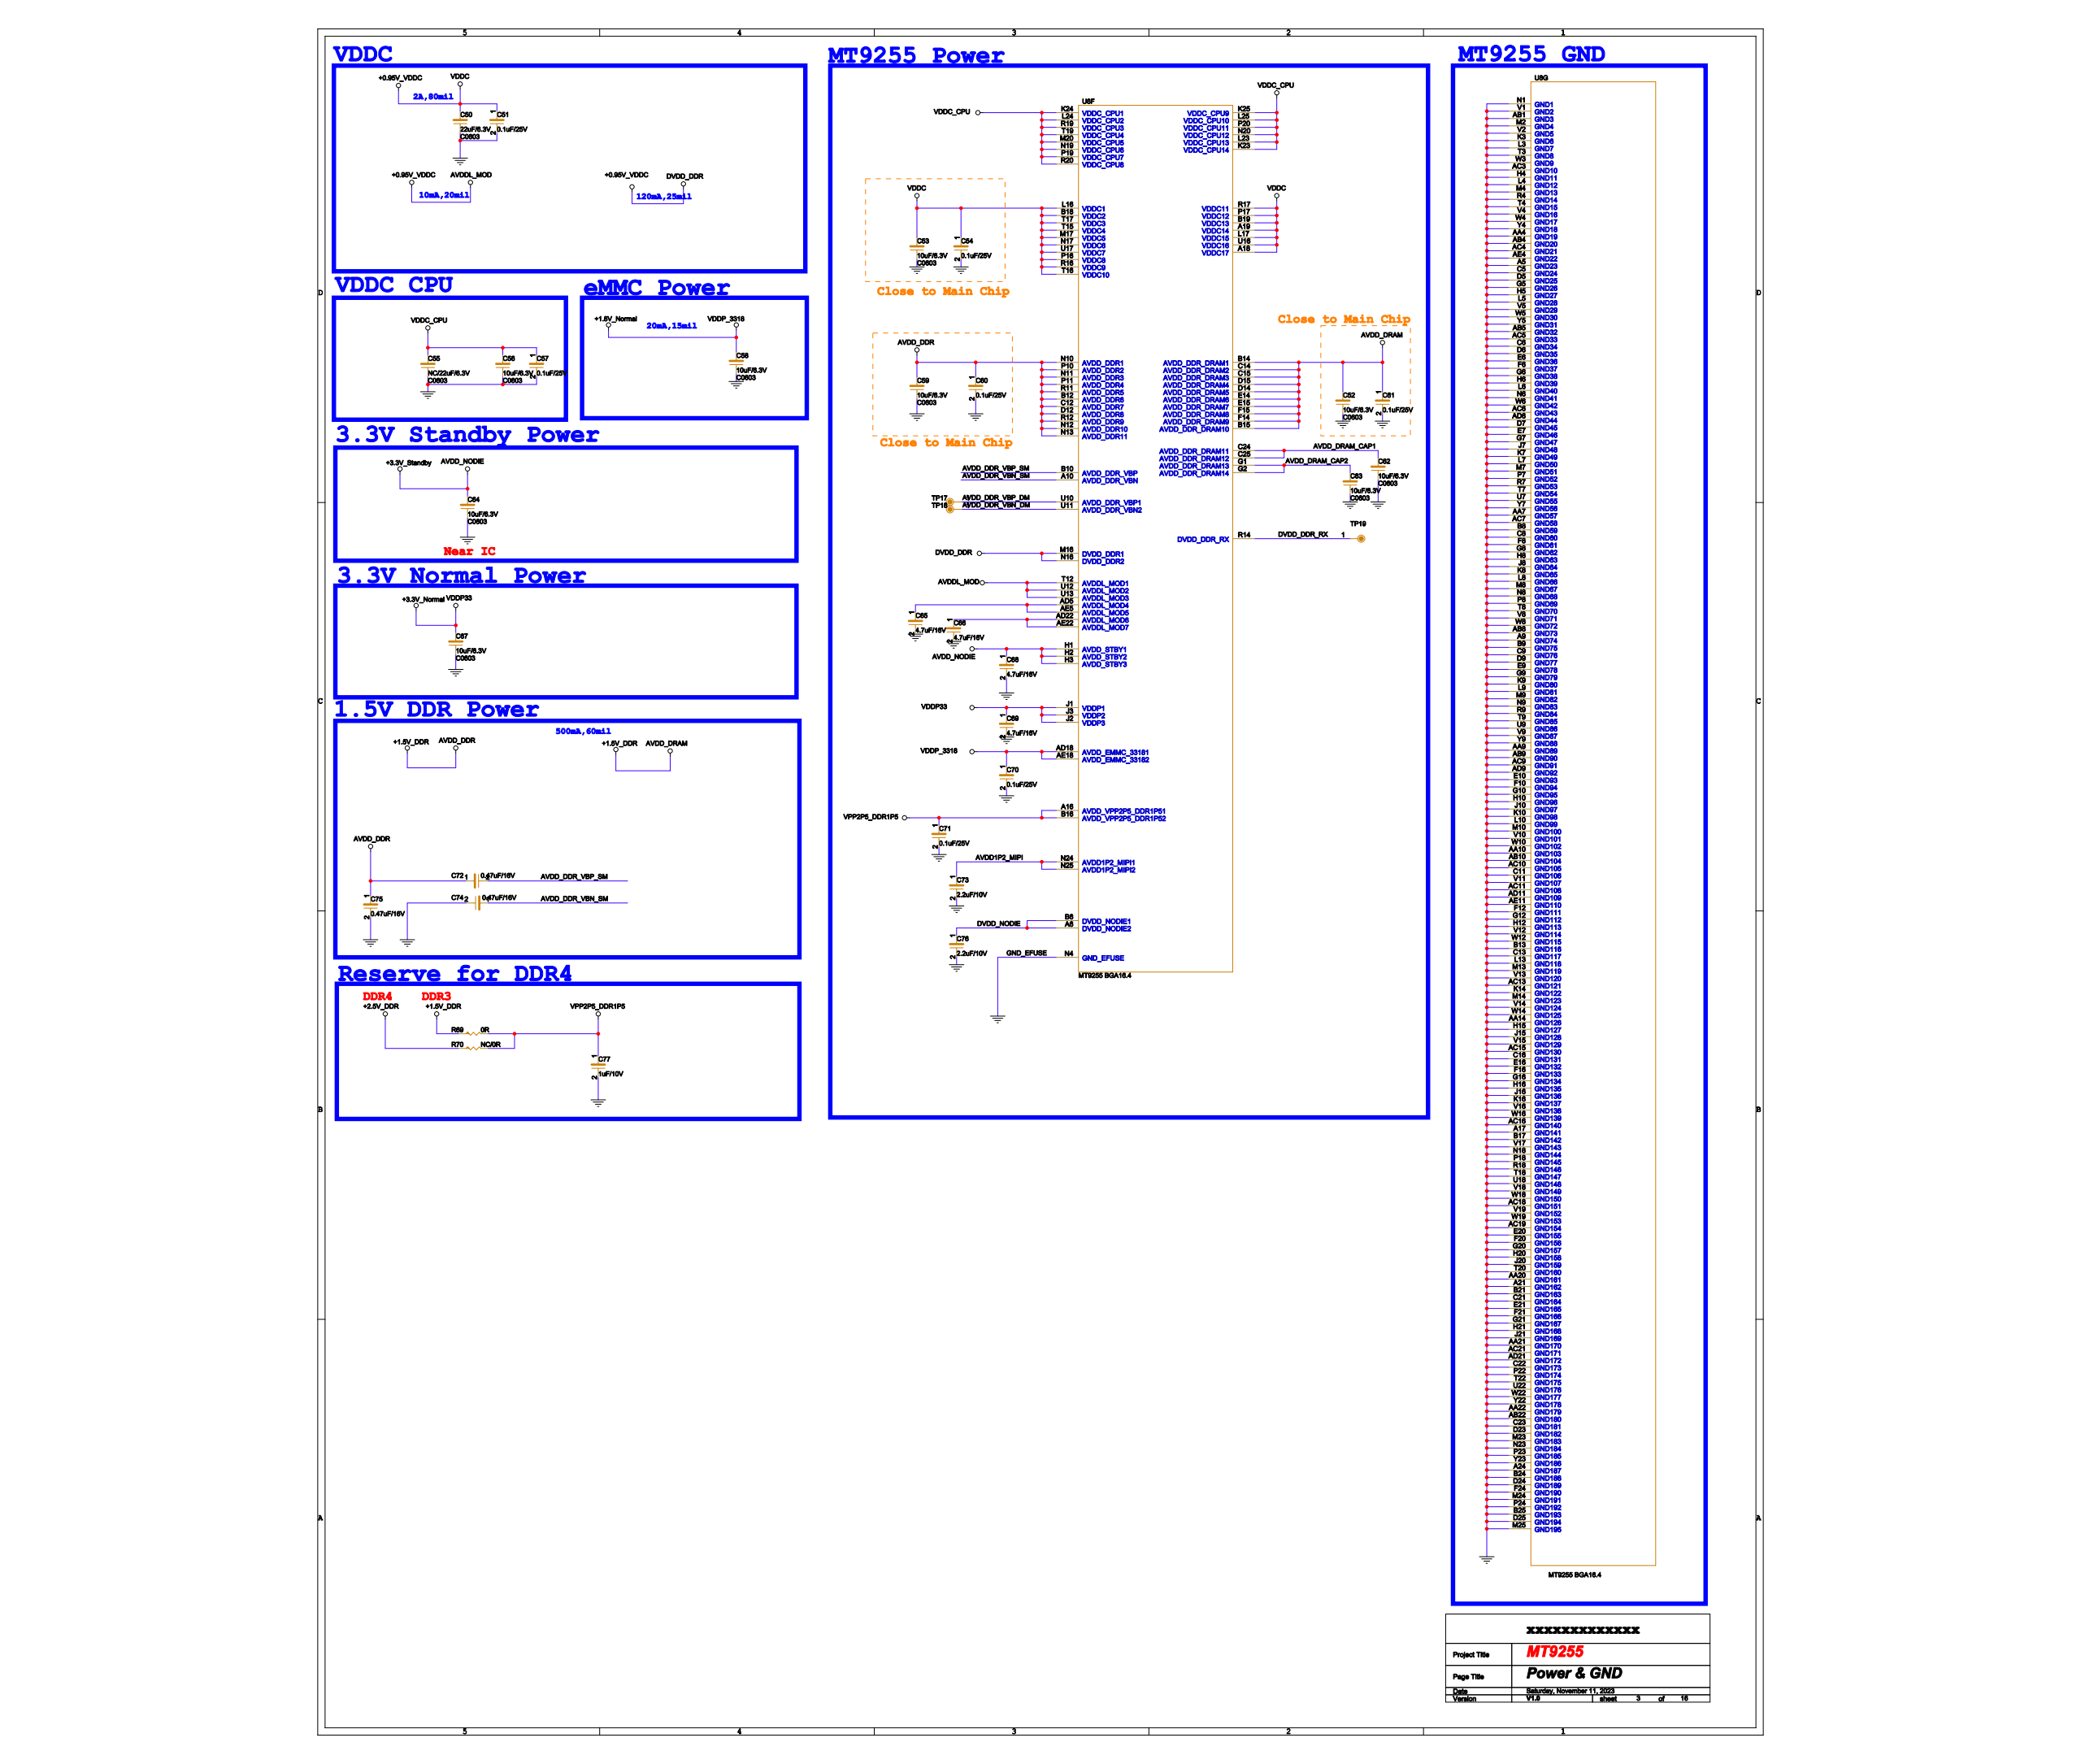Circuit board | Cadence Allegro | 1223 parts | 777 nets | one sheet of the schematic
Parts on this sheet (reference | value | footprint):
C50 | 22uF/6.3V | C0603
C51 | 0.1uF/25V | C0402
C52 | 10uF/6.3V | C0603
C53 | 10uF/6.3V | C0603
C54 | 0.1uF/25V | C0402
C55 | NC/22uF/6.3V | C0603
C56 | 10uF/6.3V | C0603
C57 | 0.1uF/25V | C0402
C58 | 10uF/6.3V | C0603
C59 | 10uF/6.3V | C0603
C60 | 0.1uF/25V | C0402
C61 | 0.1uF/25V | C0402
C62 | 10uF/6.3V | C0603
C63 | 10uF/6.3V | C0603
C64 | 10uF/6.3V | C0603
C65 | 4.7uF/16V | C0603
C66 | 4.7uF/16V | C0603
C67 | 10uF/6.3V | C0603
C68 | 4.7uF/16V | C0603
C69 | 4.7uF/16V | C0603
C70 | 0.1uF/25V | C0402
C71 | 0.1uF/25V | C0402
C72 | 0.47uF/16V | C0402
C73 | 2.2uF/10V | C0402
C74 | 0.47uF/16V | C0402
C75 | 0.47uF/16V | C0402
C76 | 2.2uF/10V | C0402
C77 | 1uF/10V | C0402
R69 | 0R | R0402
R70 | NC/0R | R0402
TP17 | DEO | TP06MM
TP18 | DEO | TP06MM
TP19 | DEO | TP06MM
U8 | MT9255 BGA16.4 | LFBGA462
U10 | EMMC_B153_2L | BGA153_13R00X11R50X0R90_2L
U16 | NTP8810 | QFN32_5X5MM
Nets of these parts (net: part-pin ...):
GND: C50-2 C51-2 C52-2 C53-2 C54-2 C55-2 C56-2 C57-2 C58-2 C59-2 C60-2 C61-2 C62-2 C63-2 C64-2 C65-2 C66-2 C67-2 C68-2 C69-2 C70-2 C71-2 C73-2 C74-2 C75-2 C76-2 C77-2 U8-A5 U8-A9 U8-A17 U8-A21 U8-A24 U8-AA4 U8-AA7 U8-AA9 U8-AA10 U8-AA14 U8-AA20 U8-AA21 U8-AA22 U8-AB1 U8-AB4 U8-AB5 U8-AB8 U8-AB9 U8-AB10 U8-AB22 U8-AC3 U8-AC4 U8-AC5 U8-AC6 U8-AC7 U8-AC9 U8-AC10 U8-AC11 U8-AC13 U8-AC15 U8-AC16 U8-AC18 U8-AC19 U8-AC21 U8-AD6 U8-AD9 U8-AD11 U8-AD21 U8-AE4 U8-AE11 U8-B8 U8-B9 U8-B13 U8-B17 U8-B21 U8-B24 U8-B25 U8-C5 U8-C6 U8-C8 U8-C9 U8-C11 U8-C13 U8-C16 U8-C21 U8-C22 U8-C23 U8-D5 U8-D6 U8-D7 U8-D9 U8-D23 U8-D24 U8-D25 U8-E6 U8-E7 U8-E9 U8-E10 U8-E16 U8-E20 U8-E21 U8-F6 U8-F8 U8-F10 U8-F12 U8-F16 U8-F20 U8-F21 U8-F24 U8-G5 U8-G6 U8-G7 U8-G8 U8-G9 U8-G10 U8-G12 U8-G16 U8-G20 U8-G21 U8-H4 U8-H5 U8-H6 U8-H8 U8-H10 U8-H12 U8-H15 U8-H16 U8-H20 U8-H21 U8-J7 U8-J8 U8-J10 U8-J15 U8-J16 U8-J20 U8-J21 U8-K3 U8-K7 U8-K8 U8-K9 U8-K10 U8-K14 U8-K16 U8-L3 U8-L4 U8-L5 U8-L6 U8-L7 U8-L8 U8-L9 U8-L10 U8-L13 U8-M2 U8-M4 U8-M7 U8-M8 U8-M9 U8-M10 U8-M13 U8-M14 U8-M23 U8-M24 U8-M25 U8-N1 U8-N4 U8-N6 U8-N8 U8-N9 U8-N18 U8-N23 U8-P7 U8-P8 U8-P18 U8-P22 U8-P23 U8-P24 U8-R4 U8-R7 U8-R9 U8-R18 U8-T3 U8-T4 U8-T7 U8-T8 U8-T9 U8-T18 U8-T20 U8-T22 U8-U7 U8-U9 U8-U18 U8-U22 U8-V1 U8-V2 U8-V4 U8-V5 U8-V8 U8-V9 U8-V10 U8-V11 U8-V12 U8-V13 U8-V14 U8-V15 U8-V16 U8-V17 U8-V18 U8-V19 U8-W3 U8-W4 U8-W5 U8-W6 U8-W8 U8-W10 U8-W12 U8-W14 U8-W16 U8-W18 U8-W19 U8-W22 U8-Y4 U8-Y5 U8-Y7 U8-Y9 U8-Y22 U8-Y23 U10-A6 U10-E7 U10-G5 U10-H10 U10-K8 U16-4
+3.3V_STANDBY: C64-1 C68-1 U8-H1 U8-H2 U8-H3
+1.5V_DDR: C52-1 C59-1 C60-1 C61-1 C72-1 C75-1 R69-1 U8-B12 U8-B14 U8-B15 U8-C12 U8-C14 U8-C15 U8-D12 U8-D14 U8-D15 U8-E14 U8-E15 U8-F14 U8-F15 U8-N10 U8-N11 U8-N12 U8-N13 U8-P10 U8-P11 U8-R11 U8-R12
+0.95V_VDDC: C50-1 C51-1 C53-1 C54-1 U8-A18 U8-A19 U8-B18 U8-B19 U8-L16 U8-L17 U8-M16 U8-M17 U8-N16 U8-N17 U8-P16 U8-P17 U8-R16 U8-R17 U8-T12 U8-T15 U8-T16 U8-T17 U8-U12 U8-U13 U8-U16 U8-U17
VDDC_CPU: C55-1 C56-1 C57-1 U8-K23 U8-K24 U8-K25 U8-L23 U8-L24 U8-L25 U8-M20 U8-N19 U8-N20 U8-P19 U8-P20 U8-R19 U8-R20 U8-T19
+3.3V_EMMC: C67-1 C69-1 U8-J1 U8-J2 U8-J3 U10-E6 U10-J10 U10-K9
+1.8V_NORMAL: C58-1 C70-1 U8-AD18 U8-AE18 U10-C6 U10-M4 U10-N4
VPP2P5_DDR1P5: C71-1 C77-1 R69-2 R70-2 U8-A16 U8-B16
+2.5V_DDR: R70-1
AVDD_DRAM_CAP1: C62-1 U8-C24 U8-C25
AVDD_DRAM_CAP2: C63-1 U8-G1 U8-G2
N185692934: C65-1 U8-AD5 U8-AE5
N185692958: C66-1 U8-AD22 U8-AE22
AVDD_DDR_VBP_SM: C72-2 U8-B10
AVDD_DDR_VBN_SM: C74-1 U8-A10
AVDD1P2_MIPI: C73-1 U8-N24 U8-N25
DVDD_NODIE: C76-1 U8-A6 U8-B6
AVDD_DDR_VBP_DM: TP17-1 U8-U10
AVDD_DDR_VBN_DM: TP18-1 U8-U11
DVDD_DDR_RX: TP19-1 U8-R14